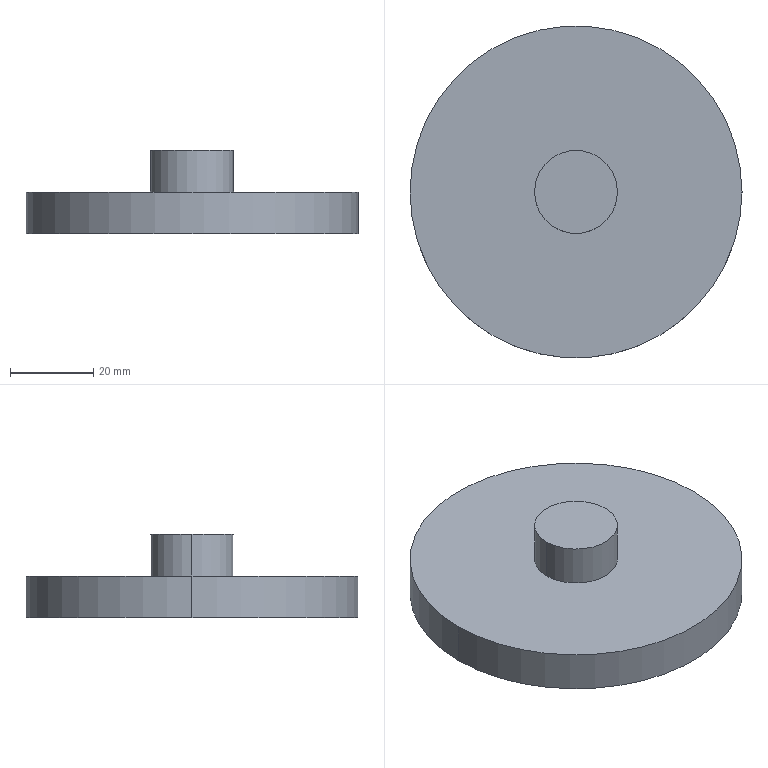Part | SolidWorks | features Extrusion 1, ICE 1 | 1 solid | 7 faces | box 80 x 80 x 20 mm | volume 53407 mm3 | cylinder 4 | plane 3 | commonest cylinder face diameters 20 x2 80 x2
STEP:
#1=CARTESIAN_POINT('',(10.,0.,20.));
#2=VERTEX_POINT('',#1);
#3=CARTESIAN_POINT('',(-10.,0.,20.));
#4=VERTEX_POINT('',#3);
#5=CARTESIAN_POINT('',(0.,0.,20.));
#6=DIRECTION('',(0.,0.,1.));
#7=DIRECTION('',(1.,0.,0.));
#8=AXIS2_PLACEMENT_3D('',#5,#6,#7);
#9=CIRCLE('',#8,10.);
#10=EDGE_CURVE('',#2,#4,#9,.T.);
#11=ORIENTED_EDGE('',*,*,#10,.F.);
#12=CARTESIAN_POINT('',(10.,0.,10.));
#13=VERTEX_POINT('',#12);
#14=CARTESIAN_POINT('',(10.,0.,20.));
#15=DIRECTION('',(0.,0.,-1.));
#16=VECTOR('',#15,1000.);
#17=LINE('',#14,#16);
#18=EDGE_CURVE('',#2,#13,#17,.T.);
#19=ORIENTED_EDGE('',*,*,#18,.T.);
#20=CARTESIAN_POINT('',(-10.,0.,10.));
#21=VERTEX_POINT('',#20);
#22=CARTESIAN_POINT('',(0.,0.,10.));
#23=DIRECTION('',(0.,0.,-1.));
#24=DIRECTION('',(1.,0.,0.));
#25=AXIS2_PLACEMENT_3D('',#22,#23,#24);
#26=CIRCLE('',#25,10.);
#27=EDGE_CURVE('',#21,#13,#26,.T.);
#28=ORIENTED_EDGE('',*,*,#27,.F.);
#29=CARTESIAN_POINT('',(-10.,0.,20.));
#30=DIRECTION('',(0.,0.,-1.));
#31=VECTOR('',#30,1000.);
#32=LINE('',#29,#31);
#33=EDGE_CURVE('',#4,#21,#32,.T.);
#34=ORIENTED_EDGE('',*,*,#33,.F.);
#35=EDGE_LOOP('',(#11,#19,#28,#34));
#36=FACE_OUTER_BOUND('',#35,.T.);
#37=CARTESIAN_POINT('',(0.,0.,20.));
#38=DIRECTION('',(0.,0.,-1.));
#39=DIRECTION('',(-1.,0.,0.));
#40=AXIS2_PLACEMENT_3D('',#37,#38,#39);
#41=CYLINDRICAL_SURFACE('',#40,10.);
#42=ADVANCED_FACE('',(#36),#41,.T.);
#43=CARTESIAN_POINT('',(40.,0.,10.));
#44=VERTEX_POINT('',#43);
#45=CARTESIAN_POINT('',(-40.,0.,10.));
#46=VERTEX_POINT('',#45);
#47=CARTESIAN_POINT('',(0.,0.,10.));
#48=DIRECTION('',(0.,0.,1.));
#49=DIRECTION('',(1.,0.,0.));
#50=AXIS2_PLACEMENT_3D('',#47,#48,#49);
#51=CIRCLE('',#50,40.);
#52=EDGE_CURVE('',#44,#46,#51,.T.);
#53=ORIENTED_EDGE('',*,*,#52,.F.);
#54=CARTESIAN_POINT('',(40.,0.,0.));
#55=VERTEX_POINT('',#54);
#56=CARTESIAN_POINT('',(40.,0.,10.));
#57=DIRECTION('',(0.,0.,-1.));
#58=VECTOR('',#57,1000.);
#59=LINE('',#56,#58);
#60=EDGE_CURVE('',#44,#55,#59,.T.);
#61=ORIENTED_EDGE('',*,*,#60,.T.);
#62=CARTESIAN_POINT('',(-40.,0.,0.));
#63=VERTEX_POINT('',#62);
#64=CARTESIAN_POINT('',(0.,0.,0.));
#65=DIRECTION('',(0.,0.,1.));
#66=DIRECTION('',(1.,0.,0.));
#67=AXIS2_PLACEMENT_3D('',#64,#65,#66);
#68=CIRCLE('',#67,40.);
#69=EDGE_CURVE('',#55,#63,#68,.T.);
#70=ORIENTED_EDGE('',*,*,#69,.T.);
#71=CARTESIAN_POINT('',(-40.,0.,10.));
#72=DIRECTION('',(0.,0.,-1.));
#73=VECTOR('',#72,1000.);
#74=LINE('',#71,#73);
#75=EDGE_CURVE('',#46,#63,#74,.T.);
#76=ORIENTED_EDGE('',*,*,#75,.F.);
#77=EDGE_LOOP('',(#53,#61,#70,#76));
#78=FACE_OUTER_BOUND('',#77,.T.);
#79=CARTESIAN_POINT('',(0.,0.,10.));
#80=DIRECTION('',(0.,0.,-1.));
#81=DIRECTION('',(-1.,0.,0.));
#82=AXIS2_PLACEMENT_3D('',#79,#80,#81);
#83=CYLINDRICAL_SURFACE('',#82,40.);
#84=ADVANCED_FACE('',(#78),#83,.T.);
#85=ORIENTED_EDGE('',*,*,#60,.F.);
#86=CARTESIAN_POINT('',(0.,0.,10.));
#87=DIRECTION('',(0.,0.,1.));
#88=DIRECTION('',(1.,0.,0.));
#89=AXIS2_PLACEMENT_3D('',#86,#87,#88);
#90=CIRCLE('',#89,40.);
#91=EDGE_CURVE('',#46,#44,#90,.T.);
#92=ORIENTED_EDGE('',*,*,#91,.F.);
#93=ORIENTED_EDGE('',*,*,#75,.T.);
#94=CARTESIAN_POINT('',(0.,0.,0.));
#95=DIRECTION('',(0.,0.,1.));
#96=DIRECTION('',(1.,0.,0.));
#97=AXIS2_PLACEMENT_3D('',#94,#95,#96);
#98=CIRCLE('',#97,40.);
#99=EDGE_CURVE('',#63,#55,#98,.T.);
#100=ORIENTED_EDGE('',*,*,#99,.T.);
#101=EDGE_LOOP('',(#85,#92,#93,#100));
#102=FACE_OUTER_BOUND('',#101,.T.);
#103=CARTESIAN_POINT('',(0.,0.,10.));
#104=DIRECTION('',(0.,0.,-1.));
#105=DIRECTION('',(-1.,0.,0.));
#106=AXIS2_PLACEMENT_3D('',#103,#104,#105);
#107=CYLINDRICAL_SURFACE('',#106,40.);
#108=ADVANCED_FACE('',(#102),#107,.T.);
#109=ORIENTED_EDGE('',*,*,#27,.T.);
#110=CARTESIAN_POINT('',(0.,0.,10.));
#111=DIRECTION('',(0.,0.,-1.));
#112=DIRECTION('',(1.,0.,0.));
#113=AXIS2_PLACEMENT_3D('',#110,#111,#112);
#114=CIRCLE('',#113,10.);
#115=EDGE_CURVE('',#13,#21,#114,.T.);
#116=ORIENTED_EDGE('',*,*,#115,.T.);
#117=EDGE_LOOP('',(#109,#116));
#118=FACE_BOUND('',#117,.T.);
#119=ORIENTED_EDGE('',*,*,#91,.T.);
#120=ORIENTED_EDGE('',*,*,#52,.T.);
#121=EDGE_LOOP('',(#119,#120));
#122=FACE_OUTER_BOUND('',#121,.T.);
#123=CARTESIAN_POINT('',(0.,0.,10.));
#124=DIRECTION('',(0.,0.,1.));
#125=DIRECTION('',(1.,0.,0.));
#126=AXIS2_PLACEMENT_3D('',#123,#124,#125);
#127=PLANE('',#126);
#128=ADVANCED_FACE('',(#118,#122),#127,.T.);
#129=ORIENTED_EDGE('',*,*,#99,.F.);
#130=ORIENTED_EDGE('',*,*,#69,.F.);
#131=EDGE_LOOP('',(#129,#130));
#132=FACE_OUTER_BOUND('',#131,.T.);
#133=CARTESIAN_POINT('',(0.,0.,0.));
#134=DIRECTION('',(0.,0.,1.));
#135=DIRECTION('',(1.,0.,0.));
#136=AXIS2_PLACEMENT_3D('',#133,#134,#135);
#137=PLANE('',#136);
#138=ADVANCED_FACE('',(#132),#137,.F.);
#139=ORIENTED_EDGE('',*,*,#18,.F.);
#140=CARTESIAN_POINT('',(0.,0.,20.));
#141=DIRECTION('',(0.,0.,1.));
#142=DIRECTION('',(1.,0.,0.));
#143=AXIS2_PLACEMENT_3D('',#140,#141,#142);
#144=CIRCLE('',#143,10.);
#145=EDGE_CURVE('',#4,#2,#144,.T.);
#146=ORIENTED_EDGE('',*,*,#145,.F.);
#147=ORIENTED_EDGE('',*,*,#33,.T.);
#148=ORIENTED_EDGE('',*,*,#115,.F.);
#149=EDGE_LOOP('',(#139,#146,#147,#148));
#150=FACE_OUTER_BOUND('',#149,.T.);
#151=CARTESIAN_POINT('',(0.,0.,20.));
#152=DIRECTION('',(0.,0.,-1.));
#153=DIRECTION('',(-1.,0.,0.));
#154=AXIS2_PLACEMENT_3D('',#151,#152,#153);
#155=CYLINDRICAL_SURFACE('',#154,10.);
#156=ADVANCED_FACE('',(#150),#155,.T.);
#157=ORIENTED_EDGE('',*,*,#145,.T.);
#158=ORIENTED_EDGE('',*,*,#10,.T.);
#159=EDGE_LOOP('',(#157,#158));
#160=FACE_OUTER_BOUND('',#159,.T.);
#161=CARTESIAN_POINT('',(0.,0.,20.));
#162=DIRECTION('',(0.,0.,1.));
#163=DIRECTION('',(1.,0.,0.));
#164=AXIS2_PLACEMENT_3D('',#161,#162,#163);
#165=PLANE('',#164);
#166=ADVANCED_FACE('',(#160),#165,.T.);
#167=CLOSED_SHELL('',(#42,#84,#108,#128,#138,#156,#166));
#168=MANIFOLD_SOLID_BREP('',#167);
#169=CARTESIAN_POINT('',(0.,0.,0.));
#170=DIRECTION('',(0.,0.,1.));
#171=DIRECTION('',(1.,0.,0.));
#172=AXIS2_PLACEMENT_3D('',#169,#170,#171);
#173=(LENGTH_UNIT()NAMED_UNIT(*)SI_UNIT(.MILLI.,.METRE.));
#174=UNCERTAINTY_MEASURE_WITH_UNIT(LENGTH_MEASURE(0.00001),#173,'','');
#175=(NAMED_UNIT(*)PLANE_ANGLE_UNIT()SI_UNIT($,.RADIAN.));
#176=(NAMED_UNIT(*)SI_UNIT($,.STERADIAN.)SOLID_ANGLE_UNIT());
#177=(GEOMETRIC_REPRESENTATION_CONTEXT(3)GLOBAL_UNCERTAINTY_ASSIGNED_CONTEXT((#174))GLOBAL_UNIT_ASSIGNED_CONTEXT((#173,#175,#176))REPRESENTATION_CONTEXT('',''));
#178=ADVANCED_BREP_SHAPE_REPRESENTATION('',(#168,#172),#177);